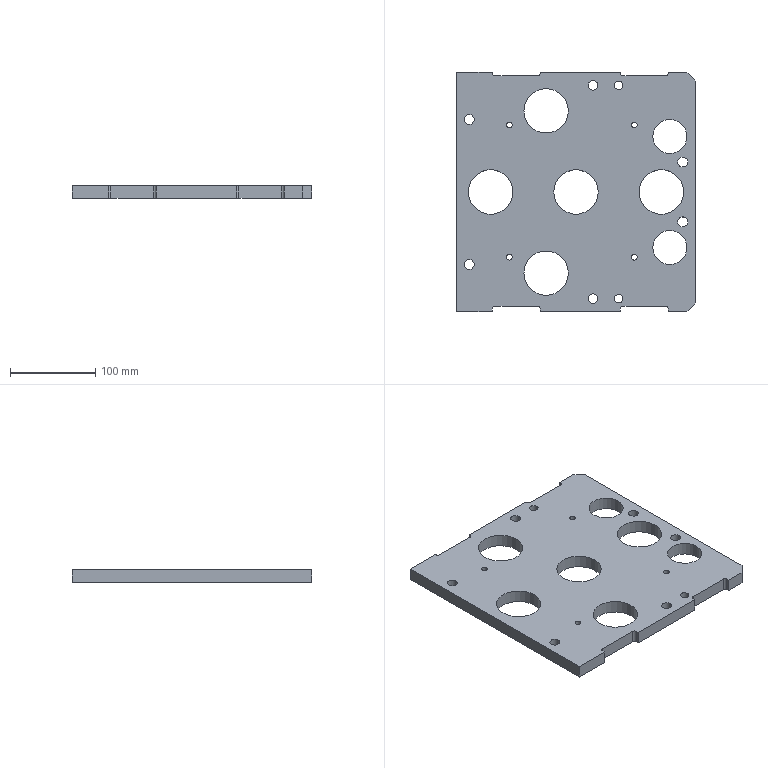Part | NX | features UB-9 2 | 1 solid | 55 faces | box 280 x 280 x 15 mm | volume 947006 mm3 | cylinder 27 | plane 24 | cone 4 | commonest cylinder face diameters 6 x8 11.507 x6 52.004 x5 6.806 x4 10 x2 40.004 x2